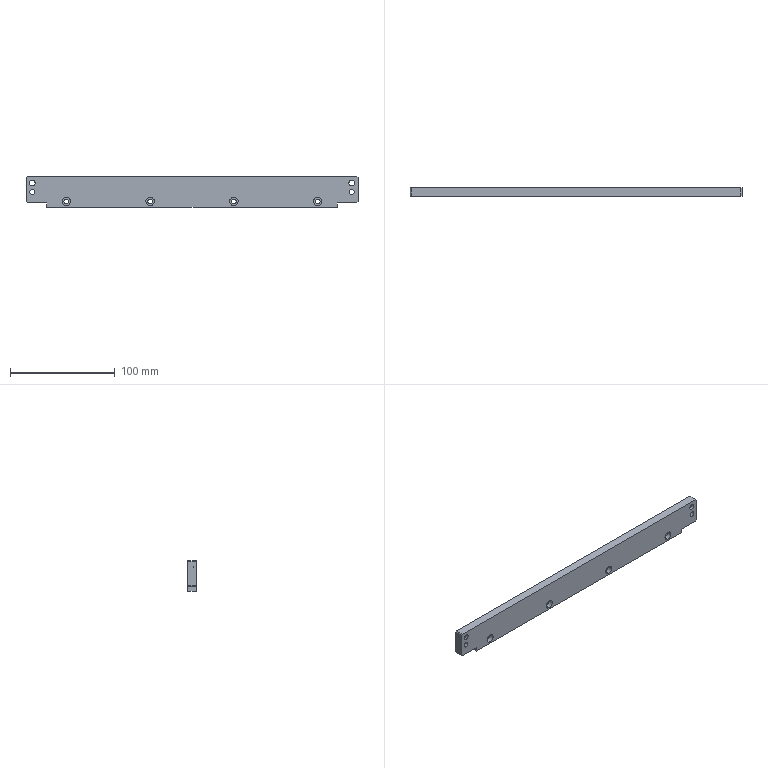Part | SolidWorks | features HoleWzd 2, ICE 2, Chamfer 1, Extrusion 1 | 1 solid | 48 faces | box 317 x 8 x 29 mm | volume 69848 mm3 | cylinder 28 | plane 20 | commonest cylinder face diameters 4.5 x8 8 x8 5 x4 5.5 x4 10 x4
STEP:
#1=CARTESIAN_POINT('',(120.,4.4,-7.));
#2=VERTEX_POINT('',#1);
#3=CARTESIAN_POINT('',(120.,4.4,-15.));
#4=VERTEX_POINT('',#3);
#5=CARTESIAN_POINT('',(120.,4.4,-11.));
#6=DIRECTION('',(0.,-1.,0.));
#7=DIRECTION('',(0.,0.,-1.));
#8=AXIS2_PLACEMENT_3D('',#5,#6,#7);
#9=CIRCLE('',#8,4.);
#10=EDGE_CURVE('',#2,#4,#9,.T.);
#11=ORIENTED_EDGE('',*,*,#10,.F.);
#12=CARTESIAN_POINT('',(120.,0.,-7.));
#13=VERTEX_POINT('',#12);
#14=CARTESIAN_POINT('',(120.,0.,-7.));
#15=DIRECTION('',(0.,-1.,0.));
#16=VECTOR('',#15,1000.);
#17=LINE('',#14,#16);
#18=EDGE_CURVE('',#2,#13,#17,.T.);
#19=ORIENTED_EDGE('',*,*,#18,.T.);
#20=CARTESIAN_POINT('',(120.,0.,-15.));
#21=VERTEX_POINT('',#20);
#22=CARTESIAN_POINT('',(120.,0.,-11.));
#23=DIRECTION('',(0.,-1.,0.));
#24=DIRECTION('',(0.,0.,-1.));
#25=AXIS2_PLACEMENT_3D('',#22,#23,#24);
#26=CIRCLE('',#25,4.);
#27=EDGE_CURVE('',#13,#21,#26,.T.);
#28=ORIENTED_EDGE('',*,*,#27,.T.);
#29=CARTESIAN_POINT('',(120.,0.,-15.));
#30=DIRECTION('',(0.,-1.,0.));
#31=VECTOR('',#30,1000.);
#32=LINE('',#29,#31);
#33=EDGE_CURVE('',#4,#21,#32,.T.);
#34=ORIENTED_EDGE('',*,*,#33,.F.);
#35=EDGE_LOOP('',(#11,#19,#28,#34));
#36=FACE_OUTER_BOUND('',#35,.T.);
#37=CARTESIAN_POINT('',(120.,0.,-11.));
#38=DIRECTION('',(0.,-1.,0.));
#39=DIRECTION('',(0.,0.,-1.));
#40=AXIS2_PLACEMENT_3D('',#37,#38,#39);
#41=CYLINDRICAL_SURFACE('',#40,4.);
#42=ADVANCED_FACE('',(#36),#41,.F.);
#43=CARTESIAN_POINT('',(120.,8.,-13.25));
#44=VERTEX_POINT('',#43);
#45=CARTESIAN_POINT('',(120.,8.,-8.75));
#46=VERTEX_POINT('',#45);
#47=CARTESIAN_POINT('',(120.,8.,-11.));
#48=DIRECTION('',(0.,1.,0.));
#49=DIRECTION('',(0.,0.,1.));
#50=AXIS2_PLACEMENT_3D('',#47,#48,#49);
#51=CIRCLE('',#50,2.25);
#52=EDGE_CURVE('',#44,#46,#51,.T.);
#53=ORIENTED_EDGE('',*,*,#52,.T.);
#54=CARTESIAN_POINT('',(120.,4.4,-8.75));
#55=VERTEX_POINT('',#54);
#56=CARTESIAN_POINT('',(120.,0.,-8.75));
#57=DIRECTION('',(0.,-1.,0.));
#58=VECTOR('',#57,1000.);
#59=LINE('',#56,#58);
#60=EDGE_CURVE('',#46,#55,#59,.T.);
#61=ORIENTED_EDGE('',*,*,#60,.T.);
#62=CARTESIAN_POINT('',(120.,4.4,-13.25));
#63=VERTEX_POINT('',#62);
#64=CARTESIAN_POINT('',(120.,4.4,-11.));
#65=DIRECTION('',(0.,-1.,0.));
#66=DIRECTION('',(0.,0.,-1.));
#67=AXIS2_PLACEMENT_3D('',#64,#65,#66);
#68=CIRCLE('',#67,2.25);
#69=EDGE_CURVE('',#55,#63,#68,.T.);
#70=ORIENTED_EDGE('',*,*,#69,.T.);
#71=CARTESIAN_POINT('',(120.,0.,-13.25));
#72=DIRECTION('',(0.,-1.,0.));
#73=VECTOR('',#72,1000.);
#74=LINE('',#71,#73);
#75=EDGE_CURVE('',#44,#63,#74,.T.);
#76=ORIENTED_EDGE('',*,*,#75,.F.);
#77=EDGE_LOOP('',(#53,#61,#70,#76));
#78=FACE_OUTER_BOUND('',#77,.T.);
#79=CARTESIAN_POINT('',(120.,0.,-11.));
#80=DIRECTION('',(0.,-1.,0.));
#81=DIRECTION('',(0.,0.,-1.));
#82=AXIS2_PLACEMENT_3D('',#79,#80,#81);
#83=CYLINDRICAL_SURFACE('',#82,2.25);
#84=ADVANCED_FACE('',(#78),#83,.F.);
#85=CARTESIAN_POINT('',(40.,4.4,-7.));
#86=VERTEX_POINT('',#85);
#87=CARTESIAN_POINT('',(40.,4.4,-15.));
#88=VERTEX_POINT('',#87);
#89=CARTESIAN_POINT('',(40.,4.4,-11.));
#90=DIRECTION('',(0.,-1.,0.));
#91=DIRECTION('',(0.,0.,-1.));
#92=AXIS2_PLACEMENT_3D('',#89,#90,#91);
#93=CIRCLE('',#92,4.);
#94=EDGE_CURVE('',#86,#88,#93,.T.);
#95=ORIENTED_EDGE('',*,*,#94,.F.);
#96=CARTESIAN_POINT('',(40.,0.,-7.));
#97=VERTEX_POINT('',#96);
#98=CARTESIAN_POINT('',(40.,0.,-7.));
#99=DIRECTION('',(0.,-1.,0.));
#100=VECTOR('',#99,1000.);
#101=LINE('',#98,#100);
#102=EDGE_CURVE('',#86,#97,#101,.T.);
#103=ORIENTED_EDGE('',*,*,#102,.T.);
#104=CARTESIAN_POINT('',(40.,0.,-15.));
#105=VERTEX_POINT('',#104);
#106=CARTESIAN_POINT('',(40.,0.,-11.));
#107=DIRECTION('',(0.,-1.,0.));
#108=DIRECTION('',(0.,0.,-1.));
#109=AXIS2_PLACEMENT_3D('',#106,#107,#108);
#110=CIRCLE('',#109,4.);
#111=EDGE_CURVE('',#97,#105,#110,.T.);
#112=ORIENTED_EDGE('',*,*,#111,.T.);
#113=CARTESIAN_POINT('',(40.,0.,-15.));
#114=DIRECTION('',(0.,-1.,0.));
#115=VECTOR('',#114,1000.);
#116=LINE('',#113,#115);
#117=EDGE_CURVE('',#88,#105,#116,.T.);
#118=ORIENTED_EDGE('',*,*,#117,.F.);
#119=EDGE_LOOP('',(#95,#103,#112,#118));
#120=FACE_OUTER_BOUND('',#119,.T.);
#121=CARTESIAN_POINT('',(40.,0.,-11.));
#122=DIRECTION('',(0.,-1.,0.));
#123=DIRECTION('',(0.,0.,-1.));
#124=AXIS2_PLACEMENT_3D('',#121,#122,#123);
#125=CYLINDRICAL_SURFACE('',#124,4.);
#126=ADVANCED_FACE('',(#120),#125,.F.);
#127=CARTESIAN_POINT('',(40.,8.,-13.25));
#128=VERTEX_POINT('',#127);
#129=CARTESIAN_POINT('',(40.,8.,-8.75));
#130=VERTEX_POINT('',#129);
#131=CARTESIAN_POINT('',(40.,8.,-11.));
#132=DIRECTION('',(0.,1.,0.));
#133=DIRECTION('',(0.,0.,1.));
#134=AXIS2_PLACEMENT_3D('',#131,#132,#133);
#135=CIRCLE('',#134,2.25);
#136=EDGE_CURVE('',#128,#130,#135,.T.);
#137=ORIENTED_EDGE('',*,*,#136,.T.);
#138=CARTESIAN_POINT('',(40.,4.4,-8.75));
#139=VERTEX_POINT('',#138);
#140=CARTESIAN_POINT('',(40.,0.,-8.75));
#141=DIRECTION('',(0.,-1.,0.));
#142=VECTOR('',#141,1000.);
#143=LINE('',#140,#142);
#144=EDGE_CURVE('',#130,#139,#143,.T.);
#145=ORIENTED_EDGE('',*,*,#144,.T.);
#146=CARTESIAN_POINT('',(40.,4.4,-13.25));
#147=VERTEX_POINT('',#146);
#148=CARTESIAN_POINT('',(40.,4.4,-11.));
#149=DIRECTION('',(0.,-1.,0.));
#150=DIRECTION('',(0.,0.,-1.));
#151=AXIS2_PLACEMENT_3D('',#148,#149,#150);
#152=CIRCLE('',#151,2.25);
#153=EDGE_CURVE('',#139,#147,#152,.T.);
#154=ORIENTED_EDGE('',*,*,#153,.T.);
#155=CARTESIAN_POINT('',(40.,0.,-13.25));
#156=DIRECTION('',(0.,-1.,0.));
#157=VECTOR('',#156,1000.);
#158=LINE('',#155,#157);
#159=EDGE_CURVE('',#128,#147,#158,.T.);
#160=ORIENTED_EDGE('',*,*,#159,.F.);
#161=EDGE_LOOP('',(#137,#145,#154,#160));
#162=FACE_OUTER_BOUND('',#161,.T.);
#163=CARTESIAN_POINT('',(40.,0.,-11.));
#164=DIRECTION('',(0.,-1.,0.));
#165=DIRECTION('',(0.,0.,-1.));
#166=AXIS2_PLACEMENT_3D('',#163,#164,#165);
#167=CYLINDRICAL_SURFACE('',#166,2.25);
#168=ADVANCED_FACE('',(#162),#167,.F.);
#169=CARTESIAN_POINT('',(-40.,4.4,-7.));
#170=VERTEX_POINT('',#169);
#171=CARTESIAN_POINT('',(-40.,4.4,-15.));
#172=VERTEX_POINT('',#171);
#173=CARTESIAN_POINT('',(-40.,4.4,-11.));
#174=DIRECTION('',(0.,-1.,0.));
#175=DIRECTION('',(0.,0.,-1.));
#176=AXIS2_PLACEMENT_3D('',#173,#174,#175);
#177=CIRCLE('',#176,4.);
#178=EDGE_CURVE('',#170,#172,#177,.T.);
#179=ORIENTED_EDGE('',*,*,#178,.F.);
#180=CARTESIAN_POINT('',(-40.,0.,-7.));
#181=VERTEX_POINT('',#180);
#182=CARTESIAN_POINT('',(-40.,0.,-7.));
#183=DIRECTION('',(0.,-1.,0.));
#184=VECTOR('',#183,1000.);
#185=LINE('',#182,#184);
#186=EDGE_CURVE('',#170,#181,#185,.T.);
#187=ORIENTED_EDGE('',*,*,#186,.T.);
#188=CARTESIAN_POINT('',(-40.,0.,-15.));
#189=VERTEX_POINT('',#188);
#190=CARTESIAN_POINT('',(-40.,0.,-11.));
#191=DIRECTION('',(0.,-1.,0.));
#192=DIRECTION('',(0.,0.,-1.));
#193=AXIS2_PLACEMENT_3D('',#190,#191,#192);
#194=CIRCLE('',#193,4.);
#195=EDGE_CURVE('',#181,#189,#194,.T.);
#196=ORIENTED_EDGE('',*,*,#195,.T.);
#197=CARTESIAN_POINT('',(-40.,0.,-15.));
#198=DIRECTION('',(0.,-1.,0.));
#199=VECTOR('',#198,1000.);
#200=LINE('',#197,#199);
#201=EDGE_CURVE('',#172,#189,#200,.T.);
#202=ORIENTED_EDGE('',*,*,#201,.F.);
#203=EDGE_LOOP('',(#179,#187,#196,#202));
#204=FACE_OUTER_BOUND('',#203,.T.);
#205=CARTESIAN_POINT('',(-40.,0.,-11.));
#206=DIRECTION('',(0.,-1.,0.));
#207=DIRECTION('',(0.,0.,-1.));
#208=AXIS2_PLACEMENT_3D('',#205,#206,#207);
#209=CYLINDRICAL_SURFACE('',#208,4.);
#210=ADVANCED_FACE('',(#204),#209,.F.);
#211=CARTESIAN_POINT('',(-40.,8.,-13.25));
#212=VERTEX_POINT('',#211);
#213=CARTESIAN_POINT('',(-40.,8.,-8.75));
#214=VERTEX_POINT('',#213);
#215=CARTESIAN_POINT('',(-40.,8.,-11.));
#216=DIRECTION('',(0.,1.,0.));
#217=DIRECTION('',(0.,0.,1.));
#218=AXIS2_PLACEMENT_3D('',#215,#216,#217);
#219=CIRCLE('',#218,2.25);
#220=EDGE_CURVE('',#212,#214,#219,.T.);
#221=ORIENTED_EDGE('',*,*,#220,.T.);
#222=CARTESIAN_POINT('',(-40.,4.4,-8.75));
#223=VERTEX_POINT('',#222);
#224=CARTESIAN_POINT('',(-40.,0.,-8.75));
#225=DIRECTION('',(0.,-1.,0.));
#226=VECTOR('',#225,1000.);
#227=LINE('',#224,#226);
#228=EDGE_CURVE('',#214,#223,#227,.T.);
#229=ORIENTED_EDGE('',*,*,#228,.T.);
#230=CARTESIAN_POINT('',(-40.,4.4,-13.25));
#231=VERTEX_POINT('',#230);
#232=CARTESIAN_POINT('',(-40.,4.4,-11.));
#233=DIRECTION('',(0.,-1.,0.));
#234=DIRECTION('',(0.,0.,-1.));
#235=AXIS2_PLACEMENT_3D('',#232,#233,#234);
#236=CIRCLE('',#235,2.25);
#237=EDGE_CURVE('',#223,#231,#236,.T.);
#238=ORIENTED_EDGE('',*,*,#237,.T.);
#239=CARTESIAN_POINT('',(-40.,0.,-13.25));
#240=DIRECTION('',(0.,-1.,0.));
#241=VECTOR('',#240,1000.);
#242=LINE('',#239,#241);
#243=EDGE_CURVE('',#212,#231,#242,.T.);
#244=ORIENTED_EDGE('',*,*,#243,.F.);
#245=EDGE_LOOP('',(#221,#229,#238,#244));
#246=FACE_OUTER_BOUND('',#245,.T.);
#247=CARTESIAN_POINT('',(-40.,0.,-11.));
#248=DIRECTION('',(0.,-1.,0.));
#249=DIRECTION('',(0.,0.,-1.));
#250=AXIS2_PLACEMENT_3D('',#247,#248,#249);
#251=CYLINDRICAL_SURFACE('',#250,2.25);
#252=ADVANCED_FACE('',(#246),#251,.F.);
#253=CARTESIAN_POINT('',(-120.,4.4,-7.));
#254=VERTEX_POINT('',#253);
#255=CARTESIAN_POINT('',(-120.,4.4,-15.));
#256=VERTEX_POINT('',#255);
#257=CARTESIAN_POINT('',(-120.,4.4,-11.));
#258=DIRECTION('',(0.,-1.,0.));
#259=DIRECTION('',(0.,0.,-1.));
#260=AXIS2_PLACEMENT_3D('',#257,#258,#259);
#261=CIRCLE('',#260,4.);
#262=EDGE_CURVE('',#254,#256,#261,.T.);
#263=ORIENTED_EDGE('',*,*,#262,.F.);
#264=CARTESIAN_POINT('',(-120.,0.,-7.));
#265=VERTEX_POINT('',#264);
#266=CARTESIAN_POINT('',(-120.,0.,-7.));
#267=DIRECTION('',(0.,-1.,0.));
#268=VECTOR('',#267,1000.);
#269=LINE('',#266,#268);
#270=EDGE_CURVE('',#254,#265,#269,.T.);
#271=ORIENTED_EDGE('',*,*,#270,.T.);
#272=CARTESIAN_POINT('',(-120.,0.,-15.));
#273=VERTEX_POINT('',#272);
#274=CARTESIAN_POINT('',(-120.,0.,-11.));
#275=DIRECTION('',(0.,-1.,0.));
#276=DIRECTION('',(0.,0.,-1.));
#277=AXIS2_PLACEMENT_3D('',#274,#275,#276);
#278=CIRCLE('',#277,4.);
#279=EDGE_CURVE('',#265,#273,#278,.T.);
#280=ORIENTED_EDGE('',*,*,#279,.T.);
#281=CARTESIAN_POINT('',(-120.,0.,-15.));
#282=DIRECTION('',(0.,-1.,0.));
#283=VECTOR('',#282,1000.);
#284=LINE('',#281,#283);
#285=EDGE_CURVE('',#256,#273,#284,.T.);
#286=ORIENTED_EDGE('',*,*,#285,.F.);
#287=EDGE_LOOP('',(#263,#271,#280,#286));
#288=FACE_OUTER_BOUND('',#287,.T.);
#289=CARTESIAN_POINT('',(-120.,0.,-11.));
#290=DIRECTION('',(0.,-1.,0.));
#291=DIRECTION('',(0.,0.,-1.));
#292=AXIS2_PLACEMENT_3D('',#289,#290,#291);
#293=CYLINDRICAL_SURFACE('',#292,4.);
#294=ADVANCED_FACE('',(#288),#293,.F.);
#295=CARTESIAN_POINT('',(-120.,8.,-13.25));
#296=VERTEX_POINT('',#295);
#297=CARTESIAN_POINT('',(-120.,8.,-8.75));
#298=VERTEX_POINT('',#297);
#299=CARTESIAN_POINT('',(-120.,8.,-11.));
#300=DIRECTION('',(0.,1.,0.));
#301=DIRECTION('',(0.,0.,1.));
#302=AXIS2_PLACEMENT_3D('',#299,#300,#301);
#303=CIRCLE('',#302,2.25);
#304=EDGE_CURVE('',#296,#298,#303,.T.);
#305=ORIENTED_EDGE('',*,*,#304,.T.);
#306=CARTESIAN_POINT('',(-120.,4.4,-8.75));
#307=VERTEX_POINT('',#306);
#308=CARTESIAN_POINT('',(-120.,0.,-8.75));
#309=DIRECTION('',(0.,-1.,0.));
#310=VECTOR('',#309,1000.);
#311=LINE('',#308,#310);
#312=EDGE_CURVE('',#298,#307,#311,.T.);
#313=ORIENTED_EDGE('',*,*,#312,.T.);
#314=CARTESIAN_POINT('',(-120.,4.4,-13.25));
#315=VERTEX_POINT('',#314);
#316=CARTESIAN_POINT('',(-120.,4.4,-11.));
#317=DIRECTION('',(0.,-1.,0.));
#318=DIRECTION('',(0.,0.,-1.));
#319=AXIS2_PLACEMENT_3D('',#316,#317,#318);
#320=CIRCLE('',#319,2.25);
#321=EDGE_CURVE('',#307,#315,#320,.T.);
#322=ORIENTED_EDGE('',*,*,#321,.T.);
#323=CARTESIAN_POINT('',(-120.,0.,-13.25));
#324=DIRECTION('',(0.,-1.,0.));
#325=VECTOR('',#324,1000.);
#326=LINE('',#323,#325);
#327=EDGE_CURVE('',#296,#315,#326,.T.);
#328=ORIENTED_EDGE('',*,*,#327,.F.);
#329=EDGE_LOOP('',(#305,#313,#322,#328));
#330=FACE_OUTER_BOUND('',#329,.T.);
#331=CARTESIAN_POINT('',(-120.,0.,-11.));
#332=DIRECTION('',(0.,-1.,0.));
#333=DIRECTION('',(0.,0.,-1.));
#334=AXIS2_PLACEMENT_3D('',#331,#332,#333);
#335=CYLINDRICAL_SURFACE('',#334,2.25);
#336=ADVANCED_FACE('',(#330),#335,.F.);
#337=CARTESIAN_POINT('',(152.5,0.,-4.5));
#338=VERTEX_POINT('',#337);
#339=CARTESIAN_POINT('',(152.5,0.,0.5));
#340=VERTEX_POINT('',#339);
#341=CARTESIAN_POINT('',(152.5,0.,-2.));
#342=DIRECTION('',(0.,1.,0.));
#343=DIRECTION('',(0.,0.,1.));
#344=AXIS2_PLACEMENT_3D('',#341,#342,#343);
#345=CIRCLE('',#344,2.5);
#346=EDGE_CURVE('',#338,#340,#345,.T.);
#347=ORIENTED_EDGE('',*,*,#346,.F.);
#348=CARTESIAN_POINT('',(152.5,8.,-4.5));
#349=VERTEX_POINT('',#348);
#350=CARTESIAN_POINT('',(152.5,0.,-4.5));
#351=DIRECTION('',(0.,1.,0.));
#352=VECTOR('',#351,1000.);
#353=LINE('',#350,#352);
#354=EDGE_CURVE('',#338,#349,#353,.T.);
#355=ORIENTED_EDGE('',*,*,#354,.T.);
#356=CARTESIAN_POINT('',(152.5,8.,0.5));
#357=VERTEX_POINT('',#356);
#358=CARTESIAN_POINT('',(152.5,8.,-2.));
#359=DIRECTION('',(0.,1.,0.));
#360=DIRECTION('',(0.,0.,1.));
#361=AXIS2_PLACEMENT_3D('',#358,#359,#360);
#362=CIRCLE('',#361,2.5);
#363=EDGE_CURVE('',#349,#357,#362,.T.);
#364=ORIENTED_EDGE('',*,*,#363,.T.);
#365=CARTESIAN_POINT('',(152.5,0.,0.5));
#366=DIRECTION('',(0.,1.,0.));
#367=VECTOR('',#366,1000.);
#368=LINE('',#365,#367);
#369=EDGE_CURVE('',#340,#357,#368,.T.);
#370=ORIENTED_EDGE('',*,*,#369,.F.);
#371=EDGE_LOOP('',(#347,#355,#364,#370));
#372=FACE_OUTER_BOUND('',#371,.T.);
#373=CARTESIAN_POINT('',(152.5,0.,-2.));
#374=DIRECTION('',(0.,1.,0.));
#375=DIRECTION('',(0.,0.,1.));
#376=AXIS2_PLACEMENT_3D('',#373,#374,#375);
#377=CYLINDRICAL_SURFACE('',#376,2.5);
#378=ADVANCED_FACE('',(#372),#377,.F.);
#379=CARTESIAN_POINT('',(-152.5,0.,-4.5));
#380=VERTEX_POINT('',#379);
#381=CARTESIAN_POINT('',(-152.5,0.,0.5));
#382=VERTEX_POINT('',#381);
#383=CARTESIAN_POINT('',(-152.5,0.,-2.));
#384=DIRECTION('',(0.,1.,0.));
#385=DIRECTION('',(0.,0.,1.));
#386=AXIS2_PLACEMENT_3D('',#383,#384,#385);
#387=CIRCLE('',#386,2.5);
#388=EDGE_CURVE('',#380,#382,#387,.T.);
#389=ORIENTED_EDGE('',*,*,#388,.F.);
#390=CARTESIAN_POINT('',(-152.5,8.,-4.5));
#391=VERTEX_POINT('',#390);
#392=CARTESIAN_POINT('',(-152.5,0.,-4.5));
#393=DIRECTION('',(0.,1.,0.));
#394=VECTOR('',#393,1000.);
#395=LINE('',#392,#394);
#396=EDGE_CURVE('',#380,#391,#395,.T.);
#397=ORIENTED_EDGE('',*,*,#396,.T.);
#398=CARTESIAN_POINT('',(-152.5,8.,0.5));
#399=VERTEX_POINT('',#398);
#400=CARTESIAN_POINT('',(-152.5,8.,-2.));
#401=DIRECTION('',(0.,1.,0.));
#402=DIRECTION('',(0.,0.,1.));
#403=AXIS2_PLACEMENT_3D('',#400,#401,#402);
#404=CIRCLE('',#403,2.5);
#405=EDGE_CURVE('',#391,#399,#404,.T.);
#406=ORIENTED_EDGE('',*,*,#405,.T.);
#407=CARTESIAN_POINT('',(-152.5,0.,0.5));
#408=DIRECTION('',(0.,1.,0.));
#409=VECTOR('',#408,1000.);
#410=LINE('',#407,#409);
#411=EDGE_CURVE('',#382,#399,#410,.T.);
#412=ORIENTED_EDGE('',*,*,#411,.F.);
#413=EDGE_LOOP('',(#389,#397,#406,#412));
#414=FACE_OUTER_BOUND('',#413,.T.);
#415=CARTESIAN_POINT('',(-152.5,0.,-2.));
#416=DIRECTION('',(0.,1.,0.));
#417=DIRECTION('',(0.,0.,1.));
#418=AXIS2_PLACEMENT_3D('',#415,#416,#417);
#419=CYLINDRICAL_SURFACE('',#418,2.5);
#420=ADVANCED_FACE('',(#414),#419,.F.);
#421=CARTESIAN_POINT('',(-152.5,2.6,1.5));
#422=VERTEX_POINT('',#421);
#423=CARTESIAN_POINT('',(-152.5,2.6,11.5));
#424=VERTEX_POINT('',#423);
#425=CARTESIAN_POINT('',(-152.5,2.6,6.5));
#426=DIRECTION('',(0.,1.,0.));
#427=DIRECTION('',(0.,0.,1.));
#428=AXIS2_PLACEMENT_3D('',#425,#426,#427);
#429=CIRCLE('',#428,5.);
#430=EDGE_CURVE('',#422,#424,#429,.T.);
#431=ORIENTED_EDGE('',*,*,#430,.F.);
#432=CARTESIAN_POINT('',(-152.5,8.,1.5));
#433=VERTEX_POINT('',#432);
#434=CARTESIAN_POINT('',(-152.5,8.,1.5));
#435=DIRECTION('',(0.,1.,0.));
#436=VECTOR('',#435,1000.);
#437=LINE('',#434,#436);
#438=EDGE_CURVE('',#422,#433,#437,.T.);
#439=ORIENTED_EDGE('',*,*,#438,.T.);
#440=CARTESIAN_POINT('',(-152.5,8.,11.5));
#441=VERTEX_POINT('',#440);
#442=CARTESIAN_POINT('',(-152.5,8.,6.5));
#443=DIRECTION('',(0.,1.,0.));
#444=DIRECTION('',(0.,0.,1.));
#445=AXIS2_PLACEMENT_3D('',#442,#443,#444);
#446=CIRCLE('',#445,5.);
#447=EDGE_CURVE('',#433,#441,#446,.T.);
#448=ORIENTED_EDGE('',*,*,#447,.T.);
#449=CARTESIAN_POINT('',(-152.5,8.,11.5));
#450=DIRECTION('',(0.,1.,0.));
#451=VECTOR('',#450,1000.);
#452=LINE('',#449,#451);
#453=EDGE_CURVE('',#424,#441,#452,.T.);
#454=ORIENTED_EDGE('',*,*,#453,.F.);
#455=EDGE_LOOP('',(#431,#439,#448,#454));
#456=FACE_OUTER_BOUND('',#455,.T.);
#457=CARTESIAN_POINT('',(-152.5,8.,6.5));
#458=DIRECTION('',(0.,1.,0.));
#459=DIRECTION('',(0.,0.,1.));
#460=AXIS2_PLACEMENT_3D('',#457,#458,#459);
#461=CYLINDRICAL_SURFACE('',#460,5.);
#462=ADVANCED_FACE('',(#456),#461,.F.);
#463=CARTESIAN_POINT('',(-152.5,0.,3.75));
#464=VERTEX_POINT('',#463);
#465=CARTESIAN_POINT('',(-152.5,0.,9.25));
#466=VERTEX_POINT('',#465);
#467=CARTESIAN_POINT('',(-152.5,0.,6.5));
#468=DIRECTION('',(0.,1.,0.));
#469=DIRECTION('',(0.,0.,1.));
#470=AXIS2_PLACEMENT_3D('',#467,#468,#469);
#471=CIRCLE('',#470,2.75);
#472=EDGE_CURVE('',#464,#466,#471,.T.);
#473=ORIENTED_EDGE('',*,*,#472,.F.);
#474=CARTESIAN_POINT('',(-152.5,2.6,3.75));
#475=VERTEX_POINT('',#474);
#476=CARTESIAN_POINT('',(-152.5,8.,3.75));
#477=DIRECTION('',(0.,1.,0.));
#478=VECTOR('',#477,1000.);
#479=LINE('',#476,#478);
#480=EDGE_CURVE('',#464,#475,#479,.T.);
#481=ORIENTED_EDGE('',*,*,#480,.T.);
#482=CARTESIAN_POINT('',(-152.5,2.6,9.25));
#483=VERTEX_POINT('',#482);
#484=CARTESIAN_POINT('',(-152.5,2.6,6.5));
#485=DIRECTION('',(0.,1.,0.));
#486=DIRECTION('',(0.,0.,1.));
#487=AXIS2_PLACEMENT_3D('',#484,#485,#486);
#488=CIRCLE('',#487,2.75);
#489=EDGE_CURVE('',#475,#483,#488,.T.);
#490=ORIENTED_EDGE('',*,*,#489,.T.);
#491=CARTESIAN_POINT('',(-152.5,8.,9.25));
#492=DIRECTION('',(0.,1.,0.));
#493=VECTOR('',#492,1000.);
#494=LINE('',#491,#493);
#495=EDGE_CURVE('',#466,#483,#494,.T.);
#496=ORIENTED_EDGE('',*,*,#495,.F.);
#497=EDGE_LOOP('',(#473,#481,#490,#496));
#498=FACE_OUTER_BOUND('',#497,.T.);
#499=CARTESIAN_POINT('',(-152.5,8.,6.5));
#500=DIRECTION('',(0.,1.,0.));
#501=DIRECTION('',(0.,0.,1.));
#502=AXIS2_PLACEMENT_3D('',#499,#500,#501);
#503=CYLINDRICAL_SURFACE('',#502,2.75);
#504=ADVANCED_FACE('',(#498),#503,.F.);
#505=CARTESIAN_POINT('',(152.5,2.6,1.5));
#506=VERTEX_POINT('',#505);
#507=CARTESIAN_POINT('',(152.5,2.6,11.5));
#508=VERTEX_POINT('',#507);
#509=CARTESIAN_POINT('',(152.5,2.6,6.5));
#510=DIRECTION('',(0.,1.,0.));
#511=DIRECTION('',(0.,0.,1.));
#512=AXIS2_PLACEMENT_3D('',#509,#510,#511);
#513=CIRCLE('',#512,5.);
#514=EDGE_CURVE('',#506,#508,#513,.T.);
#515=ORIENTED_EDGE('',*,*,#514,.F.);
#516=CARTESIAN_POINT('',(152.5,8.,1.5));
#517=VERTEX_POINT('',#516);
#518=CARTESIAN_POINT('',(152.5,8.,1.5));
#519=DIRECTION('',(0.,1.,0.));
#520=VECTOR('',#519,1000.);
#521=LINE('',#518,#520);
#522=EDGE_CURVE('',#506,#517,#521,.T.);
#523=ORIENTED_EDGE('',*,*,#522,.T.);
#524=CARTESIAN_POINT('',(152.5,8.,11.5));
#525=VERTEX_POINT('',#524);
#526=CARTESIAN_POINT('',(152.5,8.,6.5));
#527=DIRECTION('',(0.,1.,0.));
#528=DIRECTION('',(0.,0.,1.));
#529=AXIS2_PLACEMENT_3D('',#526,#527,#528);
#530=CIRCLE('',#529,5.);
#531=EDGE_CURVE('',#517,#525,#530,.T.);
#532=ORIENTED_EDGE('',*,*,#531,.T.);
#533=CARTESIAN_POINT('',(152.5,8.,11.5));
#534=DIRECTION('',(0.,1.,0.));
#535=VECTOR('',#534,1000.);
#536=LINE('',#533,#535);
#537=EDGE_CURVE('',#508,#525,#536,.T.);
#538=ORIENTED_EDGE('',*,*,#537,.F.);
#539=EDGE_LOOP('',(#515,#523,#532,#538));
#540=FACE_OUTER_BOUND('',#539,.T.);
#541=CARTESIAN_POINT('',(152.5,8.,6.5));
#542=DIRECTION('',(0.,1.,0.));
#543=DIRECTION('',(0.,0.,1.));
#544=AXIS2_PLACEMENT_3D('',#541,#542,#543);
#545=CYLINDRICAL_SURFACE('',#544,5.);
#546=ADVANCED_FACE('',(#540),#545,.F.);
#547=CARTESIAN_POINT('',(152.5,0.,3.75));
#548=VERTEX_POINT('',#547);
#549=CARTESIAN_POINT('',(152.5,0.,9.25));
#550=VERTEX_POINT('',#549);
#551=CARTESIAN_POINT('',(152.5,0.,6.5));
#552=DIRECTION('',(0.,1.,0.));
#553=DIRECTION('',(0.,0.,1.));
#554=AXIS2_PLACEMENT_3D('',#551,#552,#553);
#555=CIRCLE('',#554,2.75);
#556=EDGE_CURVE('',#548,#550,#555,.T.);
#557=ORIENTED_EDGE('',*,*,#556,.F.);
#558=CARTESIAN_POINT('',(152.5,2.6,3.75));
#559=VERTEX_POINT('',#558);
#560=CARTESIAN_POINT('',(152.5,8.,3.75));
#561=DIRECTION('',(0.,1.,0.));
#562=VECTOR('',#561,1000.);
#563=LINE('',#560,#562);
#564=EDGE_CURVE('',#548,#559,#563,.T.);
#565=ORIENTED_EDGE('',*,*,#564,.T.);
#566=CARTESIAN_POINT('',(152.5,2.6,9.25));
#567=VERTEX_POINT('',#566);
#568=CARTESIAN_POINT('',(152.5,2.6,6.5));
#569=DIRECTION('',(0.,1.,0.));
#570=DIRECTION('',(0.,0.,1.));
#571=AXIS2_PLACEMENT_3D('',#568,#569,#570);
#572=CIRCLE('',#571,2.75);
#573=EDGE_CURVE('',#559,#567,#572,.T.);
#574=ORIENTED_EDGE('',*,*,#573,.T.);
#575=CARTESIAN_POINT('',(152.5,8.,9.25));
#576=DIRECTION('',(0.,1.,0.));
#577=VECTOR('',#576,1000.);
#578=LINE('',#575,#577);
#579=EDGE_CURVE('',#550,#567,#578,.T.);
#580=ORIENTED_EDGE('',*,*,#579,.F.);
#581=EDGE_LOOP('',(#557,#565,#574,#580));
#582=FACE_OUTER_BOUND('',#581,.T.);
#583=CARTESIAN_POINT('',(152.5,8.,6.5));
#584=DIRECTION('',(0.,1.,0.));
#585=DIRECTION('',(0.,0.,1.));
#586=AXIS2_PLACEMENT_3D('',#583,#584,#585);
#587=CYLINDRICAL_SURFACE('',#586,2.75);
#588=ADVANCED_FACE('',(#582),#587,.F.);
#589=CARTESIAN_POINT('',(157.5,8.,-12.5));
#590=VERTEX_POINT('',#589);
#591=CARTESIAN_POINT('',(138.5,8.,-12.5));
#592=VERTEX_POINT('',#591);
#593=CARTESIAN_POINT('',(-158.5,8.,-12.5));
#594=DIRECTION('',(-1.,0.,0.));
#595=VECTOR('',#594,1000.);
#596=LINE('',#593,#595);
#597=EDGE_CURVE('',#590,#592,#596,.T.);
#598=ORIENTED_EDGE('',*,*,#597,.F.);
#599=CARTESIAN_POINT('',(157.5,0.,-12.5));
#600=VERTEX_POINT('',#599);
#601=CARTESIAN_POINT('',(157.5,8.,-12.5));
#602=DIRECTION('',(0.,-1.,0.));
#603=VECTOR('',#602,1000.);
#604=LINE('',#601,#603);
#605=EDGE_CURVE('',#590,#600,#604,.T.);
#606=ORIENTED_EDGE('',*,*,#605,.T.);
#607=CARTESIAN_POINT('',(138.5,0.,-12.5));
#608=VERTEX_POINT('',#607);
#609=CARTESIAN_POINT('',(-158.5,0.,-12.5));
#610=DIRECTION('',(-1.,0.,0.));
#611=VECTOR('',#610,1000.);
#612=LINE('',#609,#611);
#613=EDGE_CURVE('',#600,#608,#612,.T.);
#614=ORIENTED_EDGE('',*,*,#613,.T.);
#615=CARTESIAN_POINT('',(138.5,285.029,-12.5));
#616=DIRECTION('',(0.,-1.,0.));
#617=VECTOR('',#616,1000.);
#618=LINE('',#615,#617);
#619=EDGE_CURVE('',#592,#608,#618,.T.);
#620=ORIENTED_EDGE('',*,*,#619,.F.);
#621=EDGE_LOOP('',(#598,#606,#614,#620));
#622=FACE_OUTER_BOUND('',#621,.T.);
#623=CARTESIAN_POINT('',(-158.5,8.,-12.5));
#624=DIRECTION('',(0.,0.,1.));
#625=DIRECTION('',(1.,0.,0.));
#626=AXIS2_PLACEMENT_3D('',#623,#624,#625);
#627=PLANE('',#626);
#628=ADVANCED_FACE('',(#622),#627,.F.);
#629=CARTESIAN_POINT('',(158.5,0.,11.5));
#630=VERTEX_POINT('',#629);
#631=CARTESIAN_POINT('',(158.5,0.,-11.5));
#632=VERTEX_POINT('',#631);
#633=CARTESIAN_POINT('',(158.5,0.,-12.5));
#634=DIRECTION('',(0.,0.,-1.));
#635=VECTOR('',#634,1000.);
#636=LINE('',#633,#635);
#637=EDGE_CURVE('',#630,#632,#636,.T.);
#638=ORIENTED_EDGE('',*,*,#637,.T.);
#639=CARTESIAN_POINT('',(158.5,8.,-11.5));
#640=VERTEX_POINT('',#639);
#641=CARTESIAN_POINT('',(158.5,8.,-11.5));
#642=DIRECTION('',(0.,1.,0.));
#643=VECTOR('',#642,1000.);
#644=LINE('',#641,#643);
#645=EDGE_CURVE('',#632,#640,#644,.T.);
#646=ORIENTED_EDGE('',*,*,#645,.T.);
#647=CARTESIAN_POINT('',(158.5,8.,11.5));
#648=VERTEX_POINT('',#647);
#649=CARTESIAN_POINT('',(158.5,8.,-12.5));
#650=DIRECTION('',(0.,0.,-1.));
#651=VECTOR('',#650,1000.);
#652=LINE('',#649,#651);
#653=EDGE_CURVE('',#648,#640,#652,.T.);
#654=ORIENTED_EDGE('',*,*,#653,.F.);
#655=CARTESIAN_POINT('',(158.5,8.,11.5));
#656=DIRECTION('',(0.,-1.,0.));
#657=VECTOR('',#656,1000.);
#658=LINE('',#655,#657);
#659=EDGE_CURVE('',#648,#630,#658,.T.);
#660=ORIENTED_EDGE('',*,*,#659,.T.);
#661=EDGE_LOOP('',(#638,#646,#654,#660));
#662=FACE_OUTER_BOUND('',#661,.T.);
#663=CARTESIAN_POINT('',(158.5,8.,-12.5));
#664=DIRECTION('',(-1.,0.,0.));
#665=DIRECTION('',(0.,0.,1.));
#666=AXIS2_PLACEMENT_3D('',#663,#664,#665);
#667=PLANE('',#666);
#668=ADVANCED_FACE('',(#662),#667,.F.);
#669=CARTESIAN_POINT('',(-138.5,0.,-12.5));
#670=VERTEX_POINT('',#669);
#671=CARTESIAN_POINT('',(-157.5,0.,-12.5));
#672=VERTEX_POINT('',#671);
#673=CARTESIAN_POINT('',(-158.5,0.,-12.5));
#674=DIRECTION('',(-1.,0.,0.));
#675=VECTOR('',#674,1000.);
#676=LINE('',#673,#675);
#677=EDGE_CURVE('',#670,#672,#676,.T.);
#678=ORIENTED_EDGE('',*,*,#677,.T.);
#679=CARTESIAN_POINT('',(-157.5,8.,-12.5));
#680=VERTEX_POINT('',#679);
#681=CARTESIAN_POINT('',(-157.5,8.,-12.5));
#682=DIRECTION('',(0.,1.,0.));
#683=VECTOR('',#682,1000.);
#684=LINE('',#681,#683);
#685=EDGE_CURVE('',#672,#680,#684,.T.);
#686=ORIENTED_EDGE('',*,*,#685,.T.);
#687=CARTESIAN_POINT('',(-138.5,8.,-12.5));
#688=VERTEX_POINT('',#687);
#689=CARTESIAN_POINT('',(-158.5,8.,-12.5));
#690=DIRECTION('',(-1.,0.,0.));
#691=VECTOR('',#690,1000.);
#692=LINE('',#689,#691);
#693=EDGE_CURVE('',#688,#680,#692,.T.);
#694=ORIENTED_EDGE('',*,*,#693,.F.);
#695=CARTESIAN_POINT('',(-138.5,285.029,-12.5));
#696=DIRECTION('',(0.,-1.,0.));
#697=VECTOR('',#696,1000.);
#698=LINE('',#695,#697);
#699=EDGE_CURVE('',#688,#670,#698,.T.);
#700=ORIENTED_EDGE('',*,*,#699,.T.);
#701=EDGE_LOOP('',(#678,#686,#694,#700));
#702=FACE_OUTER_BOUND('',#701,.T.);
#703=CARTESIAN_POINT('',(-158.5,8.,-12.5));
#704=DIRECTION('',(0.,0.,1.));
#705=DIRECTION('',(1.,0.,0.));
#706=AXIS2_PLACEMENT_3D('',#703,#704,#705);
#707=PLANE('',#706);
#708=ADVANCED_FACE('',(#702),#707,.F.);
#709=CARTESIAN_POINT('',(-158.5,8.,-11.5));
#710=VERTEX_POINT('',#709);
#711=CARTESIAN_POINT('',(-158.5,8.,11.5));
#712=VERTEX_POINT('',#711);
#713=CARTESIAN_POINT('',(-158.5,8.,-12.5));
#714=DIRECTION('',(0.,0.,1.));
#715=VECTOR('',#714,1000.);
#716=LINE('',#713,#715);
#717=EDGE_CURVE('',#710,#712,#716,.T.);
#718=ORIENTED_EDGE('',*,*,#717,.F.);
#719=CARTESIAN_POINT('',(-158.5,0.,-11.5));
#720=VERTEX_POINT('',#719);
#721=CARTESIAN_POINT('',(-158.5,8.,-11.5));
#722=DIRECTION('',(0.,-1.,0.));
#723=VECTOR('',#722,1000.);
#724=LINE('',#721,#723);
#725=EDGE_CURVE('',#710,#720,#724,.T.);
#726=ORIENTED_EDGE('',*,*,#725,.T.);
#727=CARTESIAN_POINT('',(-158.5,0.,11.5));
#728=VERTEX_POINT('',#727);
#729=CARTESIAN_POINT('',(-158.5,0.,-12.5));
#730=DIRECTION('',(0.,0.,1.));
#731=VECTOR('',#730,1000.);
#732=LINE('',#729,#731);
#733=EDGE_CURVE('',#720,#728,#732,.T.);
#734=ORIENTED_EDGE('',*,*,#733,.T.);
#735=CARTESIAN_POINT('',(-158.5,8.,11.5));
#736=DIRECTION('',(0.,1.,0.));
#737=VECTOR('',#736,1000.);
#738=LINE('',#735,#737);
#739=EDGE_CURVE('',#728,#712,#738,.T.);
#740=ORIENTED_EDGE('',*,*,#739,.T.);
#741=EDGE_LOOP('',(#718,#726,#734,#740));
#742=FACE_OUTER_BOUND('',#741,.T.);
#743=CARTESIAN_POINT('',(-158.5,8.,-12.5));
#744=DIRECTION('',(1.,0.,0.));
#745=DIRECTION('',(0.,0.,-1.));
#746=AXIS2_PLACEMENT_3D('',#743,#744,#745);
#747=PLANE('',#746);
#748=ADVANCED_FACE('',(#742),#747,.F.);
#749=CARTESIAN_POINT('',(-157.5,8.,12.5));
#750=VERTEX_POINT('',#749);
#751=CARTESIAN_POINT('',(157.5,8.,12.5));
#752=VERTEX_POINT('',#751);
#753=CARTESIAN_POINT('',(-158.5,8.,12.5));
#754=DIRECTION('',(1.,0.,0.));
#755=VECTOR('',#754,1000.);
#756=LINE('',#753,#755);
#757=EDGE_CURVE('',#750,#752,#756,.T.);
#758=ORIENTED_EDGE('',*,*,#757,.F.);
#759=CARTESIAN_POINT('',(-157.5,0.,12.5));
#760=VERTEX_POINT('',#759);
#761=CARTESIAN_POINT('',(-157.5,8.,12.5));
#762=DIRECTION('',(0.,-1.,0.));
#763=VECTOR('',#762,1000.);
#764=LINE('',#761,#763);
#765=EDGE_CURVE('',#750,#760,#764,.T.);
#766=ORIENTED_EDGE('',*,*,#765,.T.);
#767=CARTESIAN_POINT('',(157.5,0.,12.5));
#768=VERTEX_POINT('',#767);
#769=CARTESIAN_POINT('',(-158.5,0.,12.5));
#770=DIRECTION('',(1.,0.,0.));
#771=VECTOR('',#770,1000.);
#772=LINE('',#769,#771);
#773=EDGE_CURVE('',#760,#768,#772,.T.);
#774=ORIENTED_EDGE('',*,*,#773,.T.);
#775=CARTESIAN_POINT('',(157.5,8.,12.5));
#776=DIRECTION('',(0.,1.,0.));
#777=VECTOR('',#776,1000.);
#778=LINE('',#775,#777);
#779=EDGE_CURVE('',#768,#752,#778,.T.);
#780=ORIENTED_EDGE('',*,*,#779,.T.);
#781=EDGE_LOOP('',(#758,#766,#774,#780));
#782=FACE_OUTER_BOUND('',#781,.T.);
#783=CARTESIAN_POINT('',(-158.5,8.,12.5));
#784=DIRECTION('',(0.,0.,-1.));
#785=DIRECTION('',(-1.,0.,0.));
#786=AXIS2_PLACEMENT_3D('',#783,#784,#785);
#787=PLANE('',#786);
#788=ADVANCED_FACE('',(#782),#787,.F.);
#789=ORIENTED_EDGE('',*,*,#52,.F.);
#790=CARTESIAN_POINT('',(120.,8.,-11.));
#791=DIRECTION('',(0.,1.,0.));
#792=DIRECTION('',(0.,0.,1.));
#793=AXIS2_PLACEMENT_3D('',#790,#791,#792);
#794=CIRCLE('',#793,2.25);
#795=EDGE_CURVE('',#46,#44,#794,.T.);
#796=ORIENTED_EDGE('',*,*,#795,.F.);
#797=EDGE_LOOP('',(#789,#796));
#798=FACE_BOUND('',#797,.T.);
#799=ORIENTED_EDGE('',*,*,#136,.F.);
#800=CARTESIAN_POINT('',(40.,8.,-11.));
#801=DIRECTION('',(0.,1.,0.));
#802=DIRECTION('',(0.,0.,1.));
#803=AXIS2_PLACEMENT_3D('',#800,#801,#802);
#804=CIRCLE('',#803,2.25);
#805=EDGE_CURVE('',#130,#128,#804,.T.);
#806=ORIENTED_EDGE('',*,*,#805,.F.);
#807=EDGE_LOOP('',(#799,#806));
#808=FACE_BOUND('',#807,.T.);
#809=ORIENTED_EDGE('',*,*,#220,.F.);
#810=CARTESIAN_POINT('',(-40.,8.,-11.));
#811=DIRECTION('',(0.,1.,0.));
#812=DIRECTION('',(0.,0.,1.));
#813=AXIS2_PLACEMENT_3D('',#810,#811,#812);
#814=CIRCLE('',#813,2.25);
#815=EDGE_CURVE('',#214,#212,#814,.T.);
#816=ORIENTED_EDGE('',*,*,#815,.F.);
#817=EDGE_LOOP('',(#809,#816));
#818=FACE_BOUND('',#817,.T.);
#819=ORIENTED_EDGE('',*,*,#304,.F.);
#820=CARTESIAN_POINT('',(-120.,8.,-11.));
#821=DIRECTION('',(0.,1.,0.));
#822=DIRECTION('',(0.,0.,1.));
#823=AXIS2_PLACEMENT_3D('',#820,#821,#822);
#824=CIRCLE('',#823,2.25);
#825=EDGE_CURVE('',#298,#296,#824,.T.);
#826=ORIENTED_EDGE('',*,*,#825,.F.);
#827=EDGE_LOOP('',(#819,#826));
#828=FACE_BOUND('',#827,.T.);
#829=CARTESIAN_POINT('',(152.5,8.,-2.));
#830=DIRECTION('',(0.,1.,0.));
#831=DIRECTION('',(0.,0.,1.));
#832=AXIS2_PLACEMENT_3D('',#829,#830,#831);
#833=CIRCLE('',#832,2.5);
#834=EDGE_CURVE('',#357,#349,#833,.T.);
#835=ORIENTED_EDGE('',*,*,#834,.F.);
#836=ORIENTED_EDGE('',*,*,#363,.F.);
#837=EDGE_LOOP('',(#835,#836));
#838=FACE_BOUND('',#837,.T.);
#839=CARTESIAN_POINT('',(-152.5,8.,-2.));
#840=DIRECTION('',(0.,1.,0.));
#841=DIRECTION('',(0.,0.,1.));
#842=AXIS2_PLACEMENT_3D('',#839,#840,#841);
#843=CIRCLE('',#842,2.5);
#844=EDGE_CURVE('',#399,#391,#843,.T.);
#845=ORIENTED_EDGE('',*,*,#844,.F.);
#846=ORIENTED_EDGE('',*,*,#405,.F.);
#847=EDGE_LOOP('',(#845,#846));
#848=FACE_BOUND('',#847,.T.);
#849=CARTESIAN_POINT('',(-152.5,8.,6.5));
#850=DIRECTION('',(0.,1.,0.));
#851=DIRECTION('',(0.,0.,1.));
#852=AXIS2_PLACEMENT_3D('',#849,#850,#851);
#853=CIRCLE('',#852,5.);
#854=EDGE_CURVE('',#441,#433,#853,.T.);
#855=ORIENTED_EDGE('',*,*,#854,.F.);
#856=ORIENTED_EDGE('',*,*,#447,.F.);
#857=EDGE_LOOP('',(#855,#856));
#858=FACE_BOUND('',#857,.T.);
#859=CARTESIAN_POINT('',(152.5,8.,6.5));
#860=DIRECTION('',(0.,1.,0.));
#861=DIRECTION('',(0.,0.,1.));
#862=AXIS2_PLACEMENT_3D('',#859,#860,#861);
#863=CIRCLE('',#862,5.);
#864=EDGE_CURVE('',#525,#517,#863,.T.);
#865=ORIENTED_EDGE('',*,*,#864,.F.);
#866=ORIENTED_EDGE('',*,*,#531,.F.);
#867=EDGE_LOOP('',(#865,#866));
#868=FACE_BOUND('',#867,.T.);
#869=ORIENTED_EDGE('',*,*,#693,.T.);
#870=CARTESIAN_POINT('',(-85.,8.,-85.));
#871=DIRECTION('',(-0.7071,0.,0.7071));
#872=VECTOR('',#871,1000.);
#873=LINE('',#870,#872);
#874=EDGE_CURVE('',#680,#710,#873,.T.);
#875=ORIENTED_EDGE('',*,*,#874,.T.);
#876=ORIENTED_EDGE('',*,*,#717,.T.);
#877=CARTESIAN_POINT('',(-85.,8.,85.));
#878=DIRECTION('',(0.7071,0.,0.7071));
#879=VECTOR('',#878,1000.);
#880=LINE('',#877,#879);
#881=EDGE_CURVE('',#712,#750,#880,.T.);
#882=ORIENTED_EDGE('',*,*,#881,.T.);
#883=ORIENTED_EDGE('',*,*,#757,.T.);
#884=CARTESIAN_POINT('',(85.,8.,85.));
#885=DIRECTION('',(0.7071,0.,-0.7071));
#886=VECTOR('',#885,1000.);
#887=LINE('',#884,#886);
#888=EDGE_CURVE('',#752,#648,#887,.T.);
#889=ORIENTED_EDGE('',*,*,#888,.T.);
#890=ORIENTED_EDGE('',*,*,#653,.T.);
#891=CARTESIAN_POINT('',(85.,8.,-85.));
#892=DIRECTION('',(-0.7071,0.,-0.7071));
#893=VECTOR('',#892,1000.);
#894=LINE('',#891,#893);
#895=EDGE_CURVE('',#640,#590,#894,.T.);
#896=ORIENTED_EDGE('',*,*,#895,.T.);
#897=ORIENTED_EDGE('',*,*,#597,.T.);
#898=CARTESIAN_POINT('',(138.5,8.,-16.5));
#899=VERTEX_POINT('',#898);
#900=CARTESIAN_POINT('',(138.5,8.,-12.5));
#901=DIRECTION('',(0.,0.,1.));
#902=VECTOR('',#901,1000.);
#903=LINE('',#900,#902);
#904=EDGE_CURVE('',#899,#592,#903,.T.);
#905=ORIENTED_EDGE('',*,*,#904,.F.);
#906=CARTESIAN_POINT('',(-138.5,8.,-16.5));
#907=VERTEX_POINT('',#906);
#908=CARTESIAN_POINT('',(-138.5,8.,-16.5));
#909=DIRECTION('',(1.,0.,0.));
#910=VECTOR('',#909,1000.);
#911=LINE('',#908,#910);
#912=EDGE_CURVE('',#907,#899,#911,.T.);
#913=ORIENTED_EDGE('',*,*,#912,.F.);
#914=CARTESIAN_POINT('',(-138.5,8.,-12.5));
#915=DIRECTION('',(0.,0.,-1.));
#916=VECTOR('',#915,1000.);
#917=LINE('',#914,#916);
#918=EDGE_CURVE('',#688,#907,#917,.T.);
#919=ORIENTED_EDGE('',*,*,#918,.F.);
#920=EDGE_LOOP('',(#869,#875,#876,#882,#883,#889,#890,#896,#897,#905,#913,#919));
#921=FACE_OUTER_BOUND('',#920,.T.);
#922=CARTESIAN_POINT('',(0.,8.,0.));
#923=DIRECTION('',(0.,1.,0.));
#924=DIRECTION('',(0.,0.,1.));
#925=AXIS2_PLACEMENT_3D('',#922,#923,#924);
#926=PLANE('',#925);
#927=ADVANCED_FACE('',(#798,#808,#818,#828,#838,#848,#858,#868,#921),#926,.T.);
#928=CARTESIAN_POINT('',(120.,0.,-11.));
#929=DIRECTION('',(0.,-1.,0.));
#930=DIRECTION('',(0.,0.,-1.));
#931=AXIS2_PLACEMENT_3D('',#928,#929,#930);
#932=CIRCLE('',#931,4.);
#933=EDGE_CURVE('',#21,#13,#932,.T.);
#934=ORIENTED_EDGE('',*,*,#933,.F.);
#935=ORIENTED_EDGE('',*,*,#27,.F.);
#936=EDGE_LOOP('',(#934,#935));
#937=FACE_BOUND('',#936,.T.);
#938=CARTESIAN_POINT('',(40.,0.,-11.));
#939=DIRECTION('',(0.,-1.,0.));
#940=DIRECTION('',(0.,0.,-1.));
#941=AXIS2_PLACEMENT_3D('',#938,#939,#940);
#942=CIRCLE('',#941,4.);
#943=EDGE_CURVE('',#105,#97,#942,.T.);
#944=ORIENTED_EDGE('',*,*,#943,.F.);
#945=ORIENTED_EDGE('',*,*,#111,.F.);
#946=EDGE_LOOP('',(#944,#945));
#947=FACE_BOUND('',#946,.T.);
#948=CARTESIAN_POINT('',(-40.,0.,-11.));
#949=DIRECTION('',(0.,-1.,0.));
#950=DIRECTION('',(0.,0.,-1.));
#951=AXIS2_PLACEMENT_3D('',#948,#949,#950);
#952=CIRCLE('',#951,4.);
#953=EDGE_CURVE('',#189,#181,#952,.T.);
#954=ORIENTED_EDGE('',*,*,#953,.F.);
#955=ORIENTED_EDGE('',*,*,#195,.F.);
#956=EDGE_LOOP('',(#954,#955));
#957=FACE_BOUND('',#956,.T.);
#958=CARTESIAN_POINT('',(-120.,0.,-11.));
#959=DIRECTION('',(0.,-1.,0.));
#960=DIRECTION('',(0.,0.,-1.));
#961=AXIS2_PLACEMENT_3D('',#958,#959,#960);
#962=CIRCLE('',#961,4.);
#963=EDGE_CURVE('',#273,#265,#962,.T.);
#964=ORIENTED_EDGE('',*,*,#963,.F.);
#965=ORIENTED_EDGE('',*,*,#279,.F.);
#966=EDGE_LOOP('',(#964,#965));
#967=FACE_BOUND('',#966,.T.);
#968=CARTESIAN_POINT('',(152.5,0.,-2.));
#969=DIRECTION('',(0.,1.,0.));
#970=DIRECTION('',(0.,0.,1.));
#971=AXIS2_PLACEMENT_3D('',#968,#969,#970);
#972=CIRCLE('',#971,2.5);
#973=EDGE_CURVE('',#340,#338,#972,.T.);
#974=ORIENTED_EDGE('',*,*,#973,.T.);
#975=ORIENTED_EDGE('',*,*,#346,.T.);
#976=EDGE_LOOP('',(#974,#975));
#977=FACE_BOUND('',#976,.T.);
#978=CARTESIAN_POINT('',(-152.5,0.,-2.));
#979=DIRECTION('',(0.,1.,0.));
#980=DIRECTION('',(0.,0.,1.));
#981=AXIS2_PLACEMENT_3D('',#978,#979,#980);
#982=CIRCLE('',#981,2.5);
#983=EDGE_CURVE('',#382,#380,#982,.T.);
#984=ORIENTED_EDGE('',*,*,#983,.T.);
#985=ORIENTED_EDGE('',*,*,#388,.T.);
#986=EDGE_LOOP('',(#984,#985));
#987=FACE_BOUND('',#986,.T.);
#988=CARTESIAN_POINT('',(-152.5,0.,6.5));
#989=DIRECTION('',(0.,1.,0.));
#990=DIRECTION('',(0.,0.,1.));
#991=AXIS2_PLACEMENT_3D('',#988,#989,#990);
#992=CIRCLE('',#991,2.75);
#993=EDGE_CURVE('',#466,#464,#992,.T.);
#994=ORIENTED_EDGE('',*,*,#993,.T.);
#995=ORIENTED_EDGE('',*,*,#472,.T.);
#996=EDGE_LOOP('',(#994,#995));
#997=FACE_BOUND('',#996,.T.);
#998=CARTESIAN_POINT('',(152.5,0.,6.5));
#999=DIRECTION('',(0.,1.,0.));
#1000=DIRECTION('',(0.,0.,1.));
#1001=AXIS2_PLACEMENT_3D('',#998,#999,#1000);
#1002=CIRCLE('',#1001,2.75);
#1003=EDGE_CURVE('',#550,#548,#1002,.T.);
#1004=ORIENTED_EDGE('',*,*,#1003,.T.);
#1005=ORIENTED_EDGE('',*,*,#556,.T.);
#1006=EDGE_LOOP('',(#1004,#1005));
#1007=FACE_BOUND('',#1006,.T.);
#1008=ORIENTED_EDGE('',*,*,#733,.F.);
#1009=CARTESIAN_POINT('',(-158.5,0.,-11.5));
#1010=DIRECTION('',(0.7071,0.,-0.7071));
#1011=VECTOR('',#1010,1000.);
#1012=LINE('',#1009,#1011);
#1013=EDGE_CURVE('',#720,#672,#1012,.T.);
#1014=ORIENTED_EDGE('',*,*,#1013,.T.);
#1015=ORIENTED_EDGE('',*,*,#677,.F.);
#1016=CARTESIAN_POINT('',(-138.5,0.,-16.5));
#1017=VERTEX_POINT('',#1016);
#1018=CARTESIAN_POINT('',(-138.5,0.,-12.5));
#1019=DIRECTION('',(0.,0.,-1.));
#1020=VECTOR('',#1019,1000.);
#1021=LINE('',#1018,#1020);
#1022=EDGE_CURVE('',#670,#1017,#1021,.T.);
#1023=ORIENTED_EDGE('',*,*,#1022,.T.);
#1024=CARTESIAN_POINT('',(138.5,0.,-16.5));
#1025=VERTEX_POINT('',#1024);
#1026=CARTESIAN_POINT('',(-138.5,0.,-16.5));
#1027=DIRECTION('',(1.,0.,0.));
#1028=VECTOR('',#1027,1000.);
#1029=LINE('',#1026,#1028);
#1030=EDGE_CURVE('',#1017,#1025,#1029,.T.);
#1031=ORIENTED_EDGE('',*,*,#1030,.T.);
#1032=CARTESIAN_POINT('',(138.5,0.,-12.5));
#1033=DIRECTION('',(0.,0.,1.));
#1034=VECTOR('',#1033,1000.);
#1035=LINE('',#1032,#1034);
#1036=EDGE_CURVE('',#1025,#608,#1035,.T.);
#1037=ORIENTED_EDGE('',*,*,#1036,.T.);
#1038=ORIENTED_EDGE('',*,*,#613,.F.);
#1039=CARTESIAN_POINT('',(157.5,0.,-12.5));
#1040=DIRECTION('',(0.7071,0.,0.7071));
#1041=VECTOR('',#1040,1000.);
#1042=LINE('',#1039,#1041);
#1043=EDGE_CURVE('',#600,#632,#1042,.T.);
#1044=ORIENTED_EDGE('',*,*,#1043,.T.);
#1045=ORIENTED_EDGE('',*,*,#637,.F.);
#1046=CARTESIAN_POINT('',(158.5,0.,11.5));
#1047=DIRECTION('',(-0.7071,0.,0.7071));
#1048=VECTOR('',#1047,1000.);
#1049=LINE('',#1046,#1048);
#1050=EDGE_CURVE('',#630,#768,#1049,.T.);
#1051=ORIENTED_EDGE('',*,*,#1050,.T.);
#1052=ORIENTED_EDGE('',*,*,#773,.F.);
#1053=CARTESIAN_POINT('',(-157.5,0.,12.5));
#1054=DIRECTION('',(-0.7071,0.,-0.7071));
#1055=VECTOR('',#1054,1000.);
#1056=LINE('',#1053,#1055);
#1057=EDGE_CURVE('',#760,#728,#1056,.T.);
#1058=ORIENTED_EDGE('',*,*,#1057,.T.);
#1059=EDGE_LOOP('',(#1008,#1014,#1015,#1023,#1031,#1037,#1038,#1044,#1045,#1051,#1052,#1058));
#1060=FACE_OUTER_BOUND('',#1059,.T.);
#1061=CARTESIAN_POINT('',(0.,0.,0.));
#1062=DIRECTION('',(0.,1.,0.));
#1063=DIRECTION('',(0.,0.,1.));
#1064=AXIS2_PLACEMENT_3D('',#1061,#1062,#1063);
#1065=PLANE('',#1064);
#1066=ADVANCED_FACE('',(#937,#947,#957,#967,#977,#987,#997,#1007,#1060),#1065,.F.);
#1067=ORIENTED_EDGE('',*,*,#564,.F.);
#1068=ORIENTED_EDGE('',*,*,#1003,.F.);
#1069=ORIENTED_EDGE('',*,*,#579,.T.);
#1070=CARTESIAN_POINT('',(152.5,2.6,6.5));
#1071=DIRECTION('',(0.,1.,0.));
#1072=DIRECTION('',(0.,0.,1.));
#1073=AXIS2_PLACEMENT_3D('',#1070,#1071,#1072);
#1074=CIRCLE('',#1073,2.75);
#1075=EDGE_CURVE('',#567,#559,#1074,.T.);
#1076=ORIENTED_EDGE('',*,*,#1075,.T.);
#1077=EDGE_LOOP('',(#1067,#1068,#1069,#1076));
#1078=FACE_OUTER_BOUND('',#1077,.T.);
#1079=CARTESIAN_POINT('',(152.5,8.,6.5));
#1080=DIRECTION('',(0.,1.,0.));
#1081=DIRECTION('',(0.,0.,1.));
#1082=AXIS2_PLACEMENT_3D('',#1079,#1080,#1081);
#1083=CYLINDRICAL_SURFACE('',#1082,2.75);
#1084=ADVANCED_FACE('',(#1078),#1083,.F.);
#1085=ORIENTED_EDGE('',*,*,#1075,.F.);
#1086=ORIENTED_EDGE('',*,*,#573,.F.);
#1087=EDGE_LOOP('',(#1085,#1086));
#1088=FACE_BOUND('',#1087,.T.);
#1089=CARTESIAN_POINT('',(152.5,2.6,6.5));
#1090=DIRECTION('',(0.,1.,0.));
#1091=DIRECTION('',(0.,0.,1.));
#1092=AXIS2_PLACEMENT_3D('',#1089,#1090,#1091);
#1093=CIRCLE('',#1092,5.);
#1094=EDGE_CURVE('',#508,#506,#1093,.T.);
#1095=ORIENTED_EDGE('',*,*,#1094,.T.);
#1096=ORIENTED_EDGE('',*,*,#514,.T.);
#1097=EDGE_LOOP('',(#1095,#1096));
#1098=FACE_OUTER_BOUND('',#1097,.T.);
#1099=CARTESIAN_POINT('',(155.25,2.6,6.5));
#1100=DIRECTION('',(0.,-1.,0.));
#1101=DIRECTION('',(0.,0.,-1.));
#1102=AXIS2_PLACEMENT_3D('',#1099,#1100,#1101);
#1103=PLANE('',#1102);
#1104=ADVANCED_FACE('',(#1088,#1098),#1103,.F.);
#1105=ORIENTED_EDGE('',*,*,#522,.F.);
#1106=ORIENTED_EDGE('',*,*,#1094,.F.);
#1107=ORIENTED_EDGE('',*,*,#537,.T.);
#1108=ORIENTED_EDGE('',*,*,#864,.T.);
#1109=EDGE_LOOP('',(#1105,#1106,#1107,#1108));
#1110=FACE_OUTER_BOUND('',#1109,.T.);
#1111=CARTESIAN_POINT('',(152.5,8.,6.5));
#1112=DIRECTION('',(0.,1.,0.));
#1113=DIRECTION('',(0.,0.,1.));
#1114=AXIS2_PLACEMENT_3D('',#1111,#1112,#1113);
#1115=CYLINDRICAL_SURFACE('',#1114,5.);
#1116=ADVANCED_FACE('',(#1110),#1115,.F.);
#1117=ORIENTED_EDGE('',*,*,#480,.F.);
#1118=ORIENTED_EDGE('',*,*,#993,.F.);
#1119=ORIENTED_EDGE('',*,*,#495,.T.);
#1120=CARTESIAN_POINT('',(-152.5,2.6,6.5));
#1121=DIRECTION('',(0.,1.,0.));
#1122=DIRECTION('',(0.,0.,1.));
#1123=AXIS2_PLACEMENT_3D('',#1120,#1121,#1122);
#1124=CIRCLE('',#1123,2.75);
#1125=EDGE_CURVE('',#483,#475,#1124,.T.);
#1126=ORIENTED_EDGE('',*,*,#1125,.T.);
#1127=EDGE_LOOP('',(#1117,#1118,#1119,#1126));
#1128=FACE_OUTER_BOUND('',#1127,.T.);
#1129=CARTESIAN_POINT('',(-152.5,8.,6.5));
#1130=DIRECTION('',(0.,1.,0.));
#1131=DIRECTION('',(0.,0.,1.));
#1132=AXIS2_PLACEMENT_3D('',#1129,#1130,#1131);
#1133=CYLINDRICAL_SURFACE('',#1132,2.75);
#1134=ADVANCED_FACE('',(#1128),#1133,.F.);
#1135=ORIENTED_EDGE('',*,*,#1125,.F.);
#1136=ORIENTED_EDGE('',*,*,#489,.F.);
#1137=EDGE_LOOP('',(#1135,#1136));
#1138=FACE_BOUND('',#1137,.T.);
#1139=CARTESIAN_POINT('',(-152.5,2.6,6.5));
#1140=DIRECTION('',(0.,1.,0.));
#1141=DIRECTION('',(0.,0.,1.));
#1142=AXIS2_PLACEMENT_3D('',#1139,#1140,#1141);
#1143=CIRCLE('',#1142,5.);
#1144=EDGE_CURVE('',#424,#422,#1143,.T.);
#1145=ORIENTED_EDGE('',*,*,#1144,.T.);
#1146=ORIENTED_EDGE('',*,*,#430,.T.);
#1147=EDGE_LOOP('',(#1145,#1146));
#1148=FACE_OUTER_BOUND('',#1147,.T.);
#1149=CARTESIAN_POINT('',(-149.75,2.6,6.5));
#1150=DIRECTION('',(0.,-1.,0.));
#1151=DIRECTION('',(0.,0.,-1.));
#1152=AXIS2_PLACEMENT_3D('',#1149,#1150,#1151);
#1153=PLANE('',#1152);
#1154=ADVANCED_FACE('',(#1138,#1148),#1153,.F.);
#1155=ORIENTED_EDGE('',*,*,#438,.F.);
#1156=ORIENTED_EDGE('',*,*,#1144,.F.);
#1157=ORIENTED_EDGE('',*,*,#453,.T.);
#1158=ORIENTED_EDGE('',*,*,#854,.T.);
#1159=EDGE_LOOP('',(#1155,#1156,#1157,#1158));
#1160=FACE_OUTER_BOUND('',#1159,.T.);
#1161=CARTESIAN_POINT('',(-152.5,8.,6.5));
#1162=DIRECTION('',(0.,1.,0.));
#1163=DIRECTION('',(0.,0.,1.));
#1164=AXIS2_PLACEMENT_3D('',#1161,#1162,#1163);
#1165=CYLINDRICAL_SURFACE('',#1164,5.);
#1166=ADVANCED_FACE('',(#1160),#1165,.F.);
#1167=ORIENTED_EDGE('',*,*,#396,.F.);
#1168=ORIENTED_EDGE('',*,*,#983,.F.);
#1169=ORIENTED_EDGE('',*,*,#411,.T.);
#1170=ORIENTED_EDGE('',*,*,#844,.T.);
#1171=EDGE_LOOP('',(#1167,#1168,#1169,#1170));
#1172=FACE_OUTER_BOUND('',#1171,.T.);
#1173=CARTESIAN_POINT('',(-152.5,0.,-2.));
#1174=DIRECTION('',(0.,1.,0.));
#1175=DIRECTION('',(0.,0.,1.));
#1176=AXIS2_PLACEMENT_3D('',#1173,#1174,#1175);
#1177=CYLINDRICAL_SURFACE('',#1176,2.5);
#1178=ADVANCED_FACE('',(#1172),#1177,.F.);
#1179=ORIENTED_EDGE('',*,*,#354,.F.);
#1180=ORIENTED_EDGE('',*,*,#973,.F.);
#1181=ORIENTED_EDGE('',*,*,#369,.T.);
#1182=ORIENTED_EDGE('',*,*,#834,.T.);
#1183=EDGE_LOOP('',(#1179,#1180,#1181,#1182));
#1184=FACE_OUTER_BOUND('',#1183,.T.);
#1185=CARTESIAN_POINT('',(152.5,0.,-2.));
#1186=DIRECTION('',(0.,1.,0.));
#1187=DIRECTION('',(0.,0.,1.));
#1188=AXIS2_PLACEMENT_3D('',#1185,#1186,#1187);
#1189=CYLINDRICAL_SURFACE('',#1188,2.5);
#1190=ADVANCED_FACE('',(#1184),#1189,.F.);
#1191=CARTESIAN_POINT('',(-138.5,285.029,-16.5));
#1192=DIRECTION('',(0.,-1.,0.));
#1193=VECTOR('',#1192,1000.);
#1194=LINE('',#1191,#1193);
#1195=EDGE_CURVE('',#907,#1017,#1194,.T.);
#1196=ORIENTED_EDGE('',*,*,#1195,.F.);
#1197=ORIENTED_EDGE('',*,*,#912,.T.);
#1198=CARTESIAN_POINT('',(138.5,285.029,-16.5));
#1199=DIRECTION('',(0.,-1.,0.));
#1200=VECTOR('',#1199,1000.);
#1201=LINE('',#1198,#1200);
#1202=EDGE_CURVE('',#899,#1025,#1201,.T.);
#1203=ORIENTED_EDGE('',*,*,#1202,.T.);
#1204=ORIENTED_EDGE('',*,*,#1030,.F.);
#1205=EDGE_LOOP('',(#1196,#1197,#1203,#1204));
#1206=FACE_OUTER_BOUND('',#1205,.T.);
#1207=CARTESIAN_POINT('',(-138.5,285.029,-16.5));
#1208=DIRECTION('',(0.,0.,-1.));
#1209=DIRECTION('',(-1.,0.,0.));
#1210=AXIS2_PLACEMENT_3D('',#1207,#1208,#1209);
#1211=PLANE('',#1210);
#1212=ADVANCED_FACE('',(#1206),#1211,.T.);
#1213=ORIENTED_EDGE('',*,*,#1202,.F.);
#1214=ORIENTED_EDGE('',*,*,#904,.T.);
#1215=ORIENTED_EDGE('',*,*,#619,.T.);
#1216=ORIENTED_EDGE('',*,*,#1036,.F.);
#1217=EDGE_LOOP('',(#1213,#1214,#1215,#1216));
#1218=FACE_OUTER_BOUND('',#1217,.T.);
#1219=CARTESIAN_POINT('',(138.5,285.029,-12.5));
#1220=DIRECTION('',(1.,0.,0.));
#1221=DIRECTION('',(0.,0.,-1.));
#1222=AXIS2_PLACEMENT_3D('',#1219,#1220,#1221);
#1223=PLANE('',#1222);
#1224=ADVANCED_FACE('',(#1218),#1223,.T.);
#1225=ORIENTED_EDGE('',*,*,#699,.F.);
#1226=ORIENTED_EDGE('',*,*,#918,.T.);
#1227=ORIENTED_EDGE('',*,*,#1195,.T.);
#1228=ORIENTED_EDGE('',*,*,#1022,.F.);
#1229=EDGE_LOOP('',(#1225,#1226,#1227,#1228));
#1230=FACE_OUTER_BOUND('',#1229,.T.);
#1231=CARTESIAN_POINT('',(-138.5,285.029,-12.5));
#1232=DIRECTION('',(-1.,0.,0.));
#1233=DIRECTION('',(0.,0.,1.));
#1234=AXIS2_PLACEMENT_3D('',#1231,#1232,#1233);
#1235=PLANE('',#1234);
#1236=ADVANCED_FACE('',(#1230),#1235,.T.);
#1237=ORIENTED_EDGE('',*,*,#312,.F.);
#1238=ORIENTED_EDGE('',*,*,#825,.T.);
#1239=ORIENTED_EDGE('',*,*,#327,.T.);
#1240=CARTESIAN_POINT('',(-120.,4.4,-11.));
#1241=DIRECTION('',(0.,-1.,0.));
#1242=DIRECTION('',(0.,0.,-1.));
#1243=AXIS2_PLACEMENT_3D('',#1240,#1241,#1242);
#1244=CIRCLE('',#1243,2.25);
#1245=EDGE_CURVE('',#315,#307,#1244,.T.);
#1246=ORIENTED_EDGE('',*,*,#1245,.T.);
#1247=EDGE_LOOP('',(#1237,#1238,#1239,#1246));
#1248=FACE_OUTER_BOUND('',#1247,.T.);
#1249=CARTESIAN_POINT('',(-120.,0.,-11.));
#1250=DIRECTION('',(0.,-1.,0.));
#1251=DIRECTION('',(0.,0.,-1.));
#1252=AXIS2_PLACEMENT_3D('',#1249,#1250,#1251);
#1253=CYLINDRICAL_SURFACE('',#1252,2.25);
#1254=ADVANCED_FACE('',(#1248),#1253,.F.);
#1255=ORIENTED_EDGE('',*,*,#1245,.F.);
#1256=ORIENTED_EDGE('',*,*,#321,.F.);
#1257=EDGE_LOOP('',(#1255,#1256));
#1258=FACE_BOUND('',#1257,.T.);
#1259=CARTESIAN_POINT('',(-120.,4.4,-11.));
#1260=DIRECTION('',(0.,-1.,0.));
#1261=DIRECTION('',(0.,0.,-1.));
#1262=AXIS2_PLACEMENT_3D('',#1259,#1260,#1261);
#1263=CIRCLE('',#1262,4.);
#1264=EDGE_CURVE('',#256,#254,#1263,.T.);
#1265=ORIENTED_EDGE('',*,*,#1264,.T.);
#1266=ORIENTED_EDGE('',*,*,#262,.T.);
#1267=EDGE_LOOP('',(#1265,#1266));
#1268=FACE_OUTER_BOUND('',#1267,.T.);
#1269=CARTESIAN_POINT('',(-117.75,4.4,-11.));
#1270=DIRECTION('',(0.,1.,0.));
#1271=DIRECTION('',(0.,0.,1.));
#1272=AXIS2_PLACEMENT_3D('',#1269,#1270,#1271);
#1273=PLANE('',#1272);
#1274=ADVANCED_FACE('',(#1258,#1268),#1273,.F.);
#1275=ORIENTED_EDGE('',*,*,#270,.F.);
#1276=ORIENTED_EDGE('',*,*,#1264,.F.);
#1277=ORIENTED_EDGE('',*,*,#285,.T.);
#1278=ORIENTED_EDGE('',*,*,#963,.T.);
#1279=EDGE_LOOP('',(#1275,#1276,#1277,#1278));
#1280=FACE_OUTER_BOUND('',#1279,.T.);
#1281=CARTESIAN_POINT('',(-120.,0.,-11.));
#1282=DIRECTION('',(0.,-1.,0.));
#1283=DIRECTION('',(0.,0.,-1.));
#1284=AXIS2_PLACEMENT_3D('',#1281,#1282,#1283);
#1285=CYLINDRICAL_SURFACE('',#1284,4.);
#1286=ADVANCED_FACE('',(#1280),#1285,.F.);
#1287=ORIENTED_EDGE('',*,*,#228,.F.);
#1288=ORIENTED_EDGE('',*,*,#815,.T.);
#1289=ORIENTED_EDGE('',*,*,#243,.T.);
#1290=CARTESIAN_POINT('',(-40.,4.4,-11.));
#1291=DIRECTION('',(0.,-1.,0.));
#1292=DIRECTION('',(0.,0.,-1.));
#1293=AXIS2_PLACEMENT_3D('',#1290,#1291,#1292);
#1294=CIRCLE('',#1293,2.25);
#1295=EDGE_CURVE('',#231,#223,#1294,.T.);
#1296=ORIENTED_EDGE('',*,*,#1295,.T.);
#1297=EDGE_LOOP('',(#1287,#1288,#1289,#1296));
#1298=FACE_OUTER_BOUND('',#1297,.T.);
#1299=CARTESIAN_POINT('',(-40.,0.,-11.));
#1300=DIRECTION('',(0.,-1.,0.));
#1301=DIRECTION('',(0.,0.,-1.));
#1302=AXIS2_PLACEMENT_3D('',#1299,#1300,#1301);
#1303=CYLINDRICAL_SURFACE('',#1302,2.25);
#1304=ADVANCED_FACE('',(#1298),#1303,.F.);
#1305=ORIENTED_EDGE('',*,*,#1295,.F.);
#1306=ORIENTED_EDGE('',*,*,#237,.F.);
#1307=EDGE_LOOP('',(#1305,#1306));
#1308=FACE_BOUND('',#1307,.T.);
#1309=CARTESIAN_POINT('',(-40.,4.4,-11.));
#1310=DIRECTION('',(0.,-1.,0.));
#1311=DIRECTION('',(0.,0.,-1.));
#1312=AXIS2_PLACEMENT_3D('',#1309,#1310,#1311);
#1313=CIRCLE('',#1312,4.);
#1314=EDGE_CURVE('',#172,#170,#1313,.T.);
#1315=ORIENTED_EDGE('',*,*,#1314,.T.);
#1316=ORIENTED_EDGE('',*,*,#178,.T.);
#1317=EDGE_LOOP('',(#1315,#1316));
#1318=FACE_OUTER_BOUND('',#1317,.T.);
#1319=CARTESIAN_POINT('',(-37.75,4.4,-11.));
#1320=DIRECTION('',(0.,1.,0.));
#1321=DIRECTION('',(0.,0.,1.));
#1322=AXIS2_PLACEMENT_3D('',#1319,#1320,#1321);
#1323=PLANE('',#1322);
#1324=ADVANCED_FACE('',(#1308,#1318),#1323,.F.);
#1325=ORIENTED_EDGE('',*,*,#186,.F.);
#1326=ORIENTED_EDGE('',*,*,#1314,.F.);
#1327=ORIENTED_EDGE('',*,*,#201,.T.);
#1328=ORIENTED_EDGE('',*,*,#953,.T.);
#1329=EDGE_LOOP('',(#1325,#1326,#1327,#1328));
#1330=FACE_OUTER_BOUND('',#1329,.T.);
#1331=CARTESIAN_POINT('',(-40.,0.,-11.));
#1332=DIRECTION('',(0.,-1.,0.));
#1333=DIRECTION('',(0.,0.,-1.));
#1334=AXIS2_PLACEMENT_3D('',#1331,#1332,#1333);
#1335=CYLINDRICAL_SURFACE('',#1334,4.);
#1336=ADVANCED_FACE('',(#1330),#1335,.F.);
#1337=ORIENTED_EDGE('',*,*,#144,.F.);
#1338=ORIENTED_EDGE('',*,*,#805,.T.);
#1339=ORIENTED_EDGE('',*,*,#159,.T.);
#1340=CARTESIAN_POINT('',(40.,4.4,-11.));
#1341=DIRECTION('',(0.,-1.,0.));
#1342=DIRECTION('',(0.,0.,-1.));
#1343=AXIS2_PLACEMENT_3D('',#1340,#1341,#1342);
#1344=CIRCLE('',#1343,2.25);
#1345=EDGE_CURVE('',#147,#139,#1344,.T.);
#1346=ORIENTED_EDGE('',*,*,#1345,.T.);
#1347=EDGE_LOOP('',(#1337,#1338,#1339,#1346));
#1348=FACE_OUTER_BOUND('',#1347,.T.);
#1349=CARTESIAN_POINT('',(40.,0.,-11.));
#1350=DIRECTION('',(0.,-1.,0.));
#1351=DIRECTION('',(0.,0.,-1.));
#1352=AXIS2_PLACEMENT_3D('',#1349,#1350,#1351);
#1353=CYLINDRICAL_SURFACE('',#1352,2.25);
#1354=ADVANCED_FACE('',(#1348),#1353,.F.);
#1355=ORIENTED_EDGE('',*,*,#1345,.F.);
#1356=ORIENTED_EDGE('',*,*,#153,.F.);
#1357=EDGE_LOOP('',(#1355,#1356));
#1358=FACE_BOUND('',#1357,.T.);
#1359=CARTESIAN_POINT('',(40.,4.4,-11.));
#1360=DIRECTION('',(0.,-1.,0.));
#1361=DIRECTION('',(0.,0.,-1.));
#1362=AXIS2_PLACEMENT_3D('',#1359,#1360,#1361);
#1363=CIRCLE('',#1362,4.);
#1364=EDGE_CURVE('',#88,#86,#1363,.T.);
#1365=ORIENTED_EDGE('',*,*,#1364,.T.);
#1366=ORIENTED_EDGE('',*,*,#94,.T.);
#1367=EDGE_LOOP('',(#1365,#1366));
#1368=FACE_OUTER_BOUND('',#1367,.T.);
#1369=CARTESIAN_POINT('',(42.25,4.4,-11.));
#1370=DIRECTION('',(0.,1.,0.));
#1371=DIRECTION('',(0.,0.,1.));
#1372=AXIS2_PLACEMENT_3D('',#1369,#1370,#1371);
#1373=PLANE('',#1372);
#1374=ADVANCED_FACE('',(#1358,#1368),#1373,.F.);
#1375=ORIENTED_EDGE('',*,*,#102,.F.);
#1376=ORIENTED_EDGE('',*,*,#1364,.F.);
#1377=ORIENTED_EDGE('',*,*,#117,.T.);
#1378=ORIENTED_EDGE('',*,*,#943,.T.);
#1379=EDGE_LOOP('',(#1375,#1376,#1377,#1378));
#1380=FACE_OUTER_BOUND('',#1379,.T.);
#1381=CARTESIAN_POINT('',(40.,0.,-11.));
#1382=DIRECTION('',(0.,-1.,0.));
#1383=DIRECTION('',(0.,0.,-1.));
#1384=AXIS2_PLACEMENT_3D('',#1381,#1382,#1383);
#1385=CYLINDRICAL_SURFACE('',#1384,4.);
#1386=ADVANCED_FACE('',(#1380),#1385,.F.);
#1387=ORIENTED_EDGE('',*,*,#60,.F.);
#1388=ORIENTED_EDGE('',*,*,#795,.T.);
#1389=ORIENTED_EDGE('',*,*,#75,.T.);
#1390=CARTESIAN_POINT('',(120.,4.4,-11.));
#1391=DIRECTION('',(0.,-1.,0.));
#1392=DIRECTION('',(0.,0.,-1.));
#1393=AXIS2_PLACEMENT_3D('',#1390,#1391,#1392);
#1394=CIRCLE('',#1393,2.25);
#1395=EDGE_CURVE('',#63,#55,#1394,.T.);
#1396=ORIENTED_EDGE('',*,*,#1395,.T.);
#1397=EDGE_LOOP('',(#1387,#1388,#1389,#1396));
#1398=FACE_OUTER_BOUND('',#1397,.T.);
#1399=CARTESIAN_POINT('',(120.,0.,-11.));
#1400=DIRECTION('',(0.,-1.,0.));
#1401=DIRECTION('',(0.,0.,-1.));
#1402=AXIS2_PLACEMENT_3D('',#1399,#1400,#1401);
#1403=CYLINDRICAL_SURFACE('',#1402,2.25);
#1404=ADVANCED_FACE('',(#1398),#1403,.F.);
#1405=ORIENTED_EDGE('',*,*,#1395,.F.);
#1406=ORIENTED_EDGE('',*,*,#69,.F.);
#1407=EDGE_LOOP('',(#1405,#1406));
#1408=FACE_BOUND('',#1407,.T.);
#1409=CARTESIAN_POINT('',(120.,4.4,-11.));
#1410=DIRECTION('',(0.,-1.,0.));
#1411=DIRECTION('',(0.,0.,-1.));
#1412=AXIS2_PLACEMENT_3D('',#1409,#1410,#1411);
#1413=CIRCLE('',#1412,4.);
#1414=EDGE_CURVE('',#4,#2,#1413,.T.);
#1415=ORIENTED_EDGE('',*,*,#1414,.T.);
#1416=ORIENTED_EDGE('',*,*,#10,.T.);
#1417=EDGE_LOOP('',(#1415,#1416));
#1418=FACE_OUTER_BOUND('',#1417,.T.);
#1419=CARTESIAN_POINT('',(122.25,4.4,-11.));
#1420=DIRECTION('',(0.,1.,0.));
#1421=DIRECTION('',(0.,0.,1.));
#1422=AXIS2_PLACEMENT_3D('',#1419,#1420,#1421);
#1423=PLANE('',#1422);
#1424=ADVANCED_FACE('',(#1408,#1418),#1423,.F.);
#1425=ORIENTED_EDGE('',*,*,#18,.F.);
#1426=ORIENTED_EDGE('',*,*,#1414,.F.);
#1427=ORIENTED_EDGE('',*,*,#33,.T.);
#1428=ORIENTED_EDGE('',*,*,#933,.T.);
#1429=EDGE_LOOP('',(#1425,#1426,#1427,#1428));
#1430=FACE_OUTER_BOUND('',#1429,.T.);
#1431=CARTESIAN_POINT('',(120.,0.,-11.));
#1432=DIRECTION('',(0.,-1.,0.));
#1433=DIRECTION('',(0.,0.,-1.));
#1434=AXIS2_PLACEMENT_3D('',#1431,#1432,#1433);
#1435=CYLINDRICAL_SURFACE('',#1434,4.);
#1436=ADVANCED_FACE('',(#1430),#1435,.F.);
#1437=ORIENTED_EDGE('',*,*,#874,.F.);
#1438=ORIENTED_EDGE('',*,*,#685,.F.);
#1439=ORIENTED_EDGE('',*,*,#1013,.F.);
#1440=ORIENTED_EDGE('',*,*,#725,.F.);
#1441=EDGE_LOOP('',(#1437,#1438,#1439,#1440));
#1442=FACE_OUTER_BOUND('',#1441,.T.);
#1443=CARTESIAN_POINT('',(-158.5,8.,-11.5));
#1444=DIRECTION('',(0.7071,0.,0.7071));
#1445=DIRECTION('',(0.,-1.,0.));
#1446=AXIS2_PLACEMENT_3D('',#1443,#1444,#1445);
#1447=PLANE('',#1446);
#1448=ADVANCED_FACE('',(#1442),#1447,.F.);
#1449=ORIENTED_EDGE('',*,*,#881,.F.);
#1450=ORIENTED_EDGE('',*,*,#739,.F.);
#1451=ORIENTED_EDGE('',*,*,#1057,.F.);
#1452=ORIENTED_EDGE('',*,*,#765,.F.);
#1453=EDGE_LOOP('',(#1449,#1450,#1451,#1452));
#1454=FACE_OUTER_BOUND('',#1453,.T.);
#1455=CARTESIAN_POINT('',(-157.5,8.,12.5));
#1456=DIRECTION('',(0.7071,0.,-0.7071));
#1457=DIRECTION('',(0.,-1.,0.));
#1458=AXIS2_PLACEMENT_3D('',#1455,#1456,#1457);
#1459=PLANE('',#1458);
#1460=ADVANCED_FACE('',(#1454),#1459,.F.);
#1461=ORIENTED_EDGE('',*,*,#895,.F.);
#1462=ORIENTED_EDGE('',*,*,#645,.F.);
#1463=ORIENTED_EDGE('',*,*,#1043,.F.);
#1464=ORIENTED_EDGE('',*,*,#605,.F.);
#1465=EDGE_LOOP('',(#1461,#1462,#1463,#1464));
#1466=FACE_OUTER_BOUND('',#1465,.T.);
#1467=CARTESIAN_POINT('',(157.5,8.,-12.5));
#1468=DIRECTION('',(-0.7071,0.,0.7071));
#1469=DIRECTION('',(0.,-1.,0.));
#1470=AXIS2_PLACEMENT_3D('',#1467,#1468,#1469);
#1471=PLANE('',#1470);
#1472=ADVANCED_FACE('',(#1466),#1471,.F.);
#1473=ORIENTED_EDGE('',*,*,#888,.F.);
#1474=ORIENTED_EDGE('',*,*,#779,.F.);
#1475=ORIENTED_EDGE('',*,*,#1050,.F.);
#1476=ORIENTED_EDGE('',*,*,#659,.F.);
#1477=EDGE_LOOP('',(#1473,#1474,#1475,#1476));
#1478=FACE_OUTER_BOUND('',#1477,.T.);
#1479=CARTESIAN_POINT('',(158.5,8.,11.5));
#1480=DIRECTION('',(-0.7071,0.,-0.7071));
#1481=DIRECTION('',(0.,-1.,0.));
#1482=AXIS2_PLACEMENT_3D('',#1479,#1480,#1481);
#1483=PLANE('',#1482);
#1484=ADVANCED_FACE('',(#1478),#1483,.F.);
#1485=CLOSED_SHELL('',(#42,#84,#126,#168,#210,#252,#294,#336,#378,#420,#462,#504,#546,#588,#628,#668,#708,#748,#788,#927,#1066,#1084,#1104,#1116,#1134,#1154,#1166,#1178,#1190,#1212,#1224,#1236,#1254,#1274,#1286,#1304,#1324,#1336,#1354,#1374,#1386,#1404,#1424,#1436,#1448,#1460,#1472,#1484));
#1486=MANIFOLD_SOLID_BREP('',#1485);
#1487=CARTESIAN_POINT('',(0.,0.,0.));
#1488=DIRECTION('',(0.,0.,1.));
#1489=DIRECTION('',(1.,0.,0.));
#1490=AXIS2_PLACEMENT_3D('',#1487,#1488,#1489);
#1491=(LENGTH_UNIT()NAMED_UNIT(*)SI_UNIT(.MILLI.,.METRE.));
#1492=UNCERTAINTY_MEASURE_WITH_UNIT(LENGTH_MEASURE(0.00001),#1491,'','');
#1493=(NAMED_UNIT(*)PLANE_ANGLE_UNIT()SI_UNIT($,.RADIAN.));
#1494=(NAMED_UNIT(*)SI_UNIT($,.STERADIAN.)SOLID_ANGLE_UNIT());
#1495=(GEOMETRIC_REPRESENTATION_CONTEXT(3)GLOBAL_UNCERTAINTY_ASSIGNED_CONTEXT((#1492))GLOBAL_UNIT_ASSIGNED_CONTEXT((#1491,#1493,#1494))REPRESENTATION_CONTEXT('',''));
#1496=ADVANCED_BREP_SHAPE_REPRESENTATION('',(#1486,#1490),#1495);